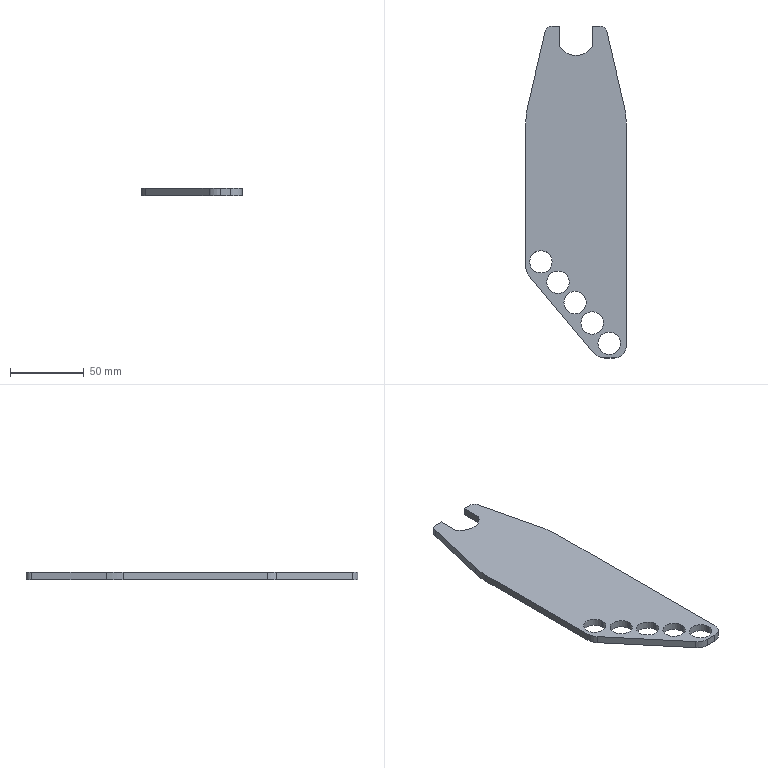Part | SolidWorks | features Fillet 5, ICE 4, Extrusion 1 | 1 solid | 30 faces | box 68 x 225 x 5 mm | volume 58604 mm3 | cylinder 18 | plane 12 | commonest cylinder face diameters 15.2 x10 10 x2 20 x2 100 x2 16 x1 26 x1
STEP:
#1=CARTESIAN_POINT('',(-8.24,-74.922,0.));
#2=VERTEX_POINT('',#1);
#3=CARTESIAN_POINT('',(6.96,-74.922,0.));
#4=VERTEX_POINT('',#3);
#5=CARTESIAN_POINT('',(-0.6404,-74.922,0.));
#6=DIRECTION('',(0.,0.,1.));
#7=DIRECTION('',(1.,0.,0.));
#8=AXIS2_PLACEMENT_3D('',#5,#6,#7);
#9=CIRCLE('',#8,7.6);
#10=EDGE_CURVE('',#2,#4,#9,.T.);
#11=ORIENTED_EDGE('',*,*,#10,.F.);
#12=CARTESIAN_POINT('',(-8.24,-74.922,5.));
#13=VERTEX_POINT('',#12);
#14=CARTESIAN_POINT('',(-8.24,-74.922,-3.));
#15=DIRECTION('',(0.,0.,1.));
#16=VECTOR('',#15,1000.);
#17=LINE('',#14,#16);
#18=EDGE_CURVE('',#2,#13,#17,.T.);
#19=ORIENTED_EDGE('',*,*,#18,.T.);
#20=CARTESIAN_POINT('',(6.96,-74.922,5.));
#21=VERTEX_POINT('',#20);
#22=CARTESIAN_POINT('',(-0.6404,-74.922,5.));
#23=DIRECTION('',(0.,0.,1.));
#24=DIRECTION('',(1.,0.,0.));
#25=AXIS2_PLACEMENT_3D('',#22,#23,#24);
#26=CIRCLE('',#25,7.6);
#27=EDGE_CURVE('',#13,#21,#26,.T.);
#28=ORIENTED_EDGE('',*,*,#27,.T.);
#29=CARTESIAN_POINT('',(6.96,-74.922,-3.));
#30=DIRECTION('',(0.,0.,1.));
#31=VECTOR('',#30,1000.);
#32=LINE('',#29,#31);
#33=EDGE_CURVE('',#4,#21,#32,.T.);
#34=ORIENTED_EDGE('',*,*,#33,.F.);
#35=EDGE_LOOP('',(#11,#19,#28,#34));
#36=FACE_OUTER_BOUND('',#35,.T.);
#37=CARTESIAN_POINT('',(-0.6404,-74.922,-3.));
#38=DIRECTION('',(0.,0.,1.));
#39=DIRECTION('',(1.,0.,0.));
#40=AXIS2_PLACEMENT_3D('',#37,#38,#39);
#41=CYLINDRICAL_SURFACE('',#40,7.6);
#42=ADVANCED_FACE('',(#36),#41,.F.);
#43=CARTESIAN_POINT('',(3.33,-88.711,0.));
#44=VERTEX_POINT('',#43);
#45=CARTESIAN_POINT('',(18.53,-88.711,0.));
#46=VERTEX_POINT('',#45);
#47=CARTESIAN_POINT('',(10.93,-88.711,0.));
#48=DIRECTION('',(0.,0.,1.));
#49=DIRECTION('',(1.,0.,0.));
#50=AXIS2_PLACEMENT_3D('',#47,#48,#49);
#51=CIRCLE('',#50,7.6);
#52=EDGE_CURVE('',#44,#46,#51,.T.);
#53=ORIENTED_EDGE('',*,*,#52,.F.);
#54=CARTESIAN_POINT('',(3.33,-88.711,5.));
#55=VERTEX_POINT('',#54);
#56=CARTESIAN_POINT('',(3.33,-88.711,-3.));
#57=DIRECTION('',(0.,0.,1.));
#58=VECTOR('',#57,1000.);
#59=LINE('',#56,#58);
#60=EDGE_CURVE('',#44,#55,#59,.T.);
#61=ORIENTED_EDGE('',*,*,#60,.T.);
#62=CARTESIAN_POINT('',(18.53,-88.711,5.));
#63=VERTEX_POINT('',#62);
#64=CARTESIAN_POINT('',(10.93,-88.711,5.));
#65=DIRECTION('',(0.,0.,1.));
#66=DIRECTION('',(1.,0.,0.));
#67=AXIS2_PLACEMENT_3D('',#64,#65,#66);
#68=CIRCLE('',#67,7.6);
#69=EDGE_CURVE('',#55,#63,#68,.T.);
#70=ORIENTED_EDGE('',*,*,#69,.T.);
#71=CARTESIAN_POINT('',(18.53,-88.711,-3.));
#72=DIRECTION('',(0.,0.,1.));
#73=VECTOR('',#72,1000.);
#74=LINE('',#71,#73);
#75=EDGE_CURVE('',#46,#63,#74,.T.);
#76=ORIENTED_EDGE('',*,*,#75,.F.);
#77=EDGE_LOOP('',(#53,#61,#70,#76));
#78=FACE_OUTER_BOUND('',#77,.T.);
#79=CARTESIAN_POINT('',(10.93,-88.711,-3.));
#80=DIRECTION('',(0.,0.,1.));
#81=DIRECTION('',(1.,0.,0.));
#82=AXIS2_PLACEMENT_3D('',#79,#80,#81);
#83=CYLINDRICAL_SURFACE('',#82,7.6);
#84=ADVANCED_FACE('',(#78),#83,.F.);
#85=CARTESIAN_POINT('',(-31.381,-47.345,0.));
#86=VERTEX_POINT('',#85);
#87=CARTESIAN_POINT('',(-16.181,-47.345,0.));
#88=VERTEX_POINT('',#87);
#89=CARTESIAN_POINT('',(-23.781,-47.345,0.));
#90=DIRECTION('',(0.,0.,1.));
#91=DIRECTION('',(1.,0.,0.));
#92=AXIS2_PLACEMENT_3D('',#89,#90,#91);
#93=CIRCLE('',#92,7.6);
#94=EDGE_CURVE('',#86,#88,#93,.T.);
#95=ORIENTED_EDGE('',*,*,#94,.F.);
#96=CARTESIAN_POINT('',(-31.381,-47.345,5.));
#97=VERTEX_POINT('',#96);
#98=CARTESIAN_POINT('',(-31.381,-47.345,-3.));
#99=DIRECTION('',(0.,0.,1.));
#100=VECTOR('',#99,1000.);
#101=LINE('',#98,#100);
#102=EDGE_CURVE('',#86,#97,#101,.T.);
#103=ORIENTED_EDGE('',*,*,#102,.T.);
#104=CARTESIAN_POINT('',(-16.181,-47.345,5.));
#105=VERTEX_POINT('',#104);
#106=CARTESIAN_POINT('',(-23.781,-47.345,5.));
#107=DIRECTION('',(0.,0.,1.));
#108=DIRECTION('',(1.,0.,0.));
#109=AXIS2_PLACEMENT_3D('',#106,#107,#108);
#110=CIRCLE('',#109,7.6);
#111=EDGE_CURVE('',#97,#105,#110,.T.);
#112=ORIENTED_EDGE('',*,*,#111,.T.);
#113=CARTESIAN_POINT('',(-16.181,-47.345,-3.));
#114=DIRECTION('',(0.,0.,1.));
#115=VECTOR('',#114,1000.);
#116=LINE('',#113,#115);
#117=EDGE_CURVE('',#88,#105,#116,.T.);
#118=ORIENTED_EDGE('',*,*,#117,.F.);
#119=EDGE_LOOP('',(#95,#103,#112,#118));
#120=FACE_OUTER_BOUND('',#119,.T.);
#121=CARTESIAN_POINT('',(-23.781,-47.345,-3.));
#122=DIRECTION('',(0.,0.,1.));
#123=DIRECTION('',(1.,0.,0.));
#124=AXIS2_PLACEMENT_3D('',#121,#122,#123);
#125=CYLINDRICAL_SURFACE('',#124,7.6);
#126=ADVANCED_FACE('',(#120),#125,.F.);
#127=CARTESIAN_POINT('',(-19.811,-61.134,0.));
#128=VERTEX_POINT('',#127);
#129=CARTESIAN_POINT('',(-4.611,-61.134,0.));
#130=VERTEX_POINT('',#129);
#131=CARTESIAN_POINT('',(-12.211,-61.134,0.));
#132=DIRECTION('',(0.,0.,1.));
#133=DIRECTION('',(1.,0.,0.));
#134=AXIS2_PLACEMENT_3D('',#131,#132,#133);
#135=CIRCLE('',#134,7.6);
#136=EDGE_CURVE('',#128,#130,#135,.T.);
#137=ORIENTED_EDGE('',*,*,#136,.F.);
#138=CARTESIAN_POINT('',(-19.811,-61.134,5.));
#139=VERTEX_POINT('',#138);
#140=CARTESIAN_POINT('',(-19.811,-61.134,-3.));
#141=DIRECTION('',(0.,0.,1.));
#142=VECTOR('',#141,1000.);
#143=LINE('',#140,#142);
#144=EDGE_CURVE('',#128,#139,#143,.T.);
#145=ORIENTED_EDGE('',*,*,#144,.T.);
#146=CARTESIAN_POINT('',(-4.611,-61.134,5.));
#147=VERTEX_POINT('',#146);
#148=CARTESIAN_POINT('',(-12.211,-61.134,5.));
#149=DIRECTION('',(0.,0.,1.));
#150=DIRECTION('',(1.,0.,0.));
#151=AXIS2_PLACEMENT_3D('',#148,#149,#150);
#152=CIRCLE('',#151,7.6);
#153=EDGE_CURVE('',#139,#147,#152,.T.);
#154=ORIENTED_EDGE('',*,*,#153,.T.);
#155=CARTESIAN_POINT('',(-4.611,-61.134,-3.));
#156=DIRECTION('',(0.,0.,1.));
#157=VECTOR('',#156,1000.);
#158=LINE('',#155,#157);
#159=EDGE_CURVE('',#130,#147,#158,.T.);
#160=ORIENTED_EDGE('',*,*,#159,.F.);
#161=EDGE_LOOP('',(#137,#145,#154,#160));
#162=FACE_OUTER_BOUND('',#161,.T.);
#163=CARTESIAN_POINT('',(-12.211,-61.134,-3.));
#164=DIRECTION('',(0.,0.,1.));
#165=DIRECTION('',(1.,0.,0.));
#166=AXIS2_PLACEMENT_3D('',#163,#164,#165);
#167=CYLINDRICAL_SURFACE('',#166,7.6);
#168=ADVANCED_FACE('',(#162),#167,.F.);
#169=CARTESIAN_POINT('',(14.9,-102.5,0.));
#170=VERTEX_POINT('',#169);
#171=CARTESIAN_POINT('',(30.1,-102.5,0.));
#172=VERTEX_POINT('',#171);
#173=CARTESIAN_POINT('',(22.5,-102.5,0.));
#174=DIRECTION('',(0.,0.,1.));
#175=DIRECTION('',(1.,0.,0.));
#176=AXIS2_PLACEMENT_3D('',#173,#174,#175);
#177=CIRCLE('',#176,7.6);
#178=EDGE_CURVE('',#170,#172,#177,.T.);
#179=ORIENTED_EDGE('',*,*,#178,.F.);
#180=CARTESIAN_POINT('',(14.9,-102.5,5.));
#181=VERTEX_POINT('',#180);
#182=CARTESIAN_POINT('',(14.9,-102.5,-3.));
#183=DIRECTION('',(0.,0.,1.));
#184=VECTOR('',#183,1000.);
#185=LINE('',#182,#184);
#186=EDGE_CURVE('',#170,#181,#185,.T.);
#187=ORIENTED_EDGE('',*,*,#186,.T.);
#188=CARTESIAN_POINT('',(30.1,-102.5,5.));
#189=VERTEX_POINT('',#188);
#190=CARTESIAN_POINT('',(22.5,-102.5,5.));
#191=DIRECTION('',(0.,0.,1.));
#192=DIRECTION('',(1.,0.,0.));
#193=AXIS2_PLACEMENT_3D('',#190,#191,#192);
#194=CIRCLE('',#193,7.6);
#195=EDGE_CURVE('',#181,#189,#194,.T.);
#196=ORIENTED_EDGE('',*,*,#195,.T.);
#197=CARTESIAN_POINT('',(30.1,-102.5,-3.));
#198=DIRECTION('',(0.,0.,1.));
#199=VECTOR('',#198,1000.);
#200=LINE('',#197,#199);
#201=EDGE_CURVE('',#172,#189,#200,.T.);
#202=ORIENTED_EDGE('',*,*,#201,.F.);
#203=EDGE_LOOP('',(#179,#187,#196,#202));
#204=FACE_OUTER_BOUND('',#203,.T.);
#205=CARTESIAN_POINT('',(22.5,-102.5,-3.));
#206=DIRECTION('',(0.,0.,1.));
#207=DIRECTION('',(1.,0.,0.));
#208=AXIS2_PLACEMENT_3D('',#205,#206,#207);
#209=CYLINDRICAL_SURFACE('',#208,7.6);
#210=ADVANCED_FACE('',(#204),#209,.F.);
#211=CARTESIAN_POINT('',(16.032,112.5,5.));
#212=VERTEX_POINT('',#211);
#213=CARTESIAN_POINT('',(11.,112.5,5.));
#214=VERTEX_POINT('',#213);
#215=CARTESIAN_POINT('',(-34.,112.5,5.));
#216=DIRECTION('',(-1.,0.,0.));
#217=VECTOR('',#216,1000.);
#218=LINE('',#215,#217);
#219=EDGE_CURVE('',#212,#214,#218,.T.);
#220=ORIENTED_EDGE('',*,*,#219,.F.);
#221=CARTESIAN_POINT('',(16.032,112.5,0.));
#222=VERTEX_POINT('',#221);
#223=CARTESIAN_POINT('',(16.032,112.5,5.));
#224=DIRECTION('',(0.,0.,-1.));
#225=VECTOR('',#224,1000.);
#226=LINE('',#223,#225);
#227=EDGE_CURVE('',#212,#222,#226,.T.);
#228=ORIENTED_EDGE('',*,*,#227,.T.);
#229=CARTESIAN_POINT('',(11.,112.5,0.));
#230=VERTEX_POINT('',#229);
#231=CARTESIAN_POINT('',(-34.,112.5,0.));
#232=DIRECTION('',(-1.,0.,0.));
#233=VECTOR('',#232,1000.);
#234=LINE('',#231,#233);
#235=EDGE_CURVE('',#222,#230,#234,.T.);
#236=ORIENTED_EDGE('',*,*,#235,.T.);
#237=CARTESIAN_POINT('',(11.,112.5,-3.));
#238=DIRECTION('',(0.,0.,1.));
#239=VECTOR('',#238,1000.);
#240=LINE('',#237,#239);
#241=EDGE_CURVE('',#230,#214,#240,.T.);
#242=ORIENTED_EDGE('',*,*,#241,.T.);
#243=EDGE_LOOP('',(#220,#228,#236,#242));
#244=FACE_OUTER_BOUND('',#243,.T.);
#245=CARTESIAN_POINT('',(-34.,112.5,5.));
#246=DIRECTION('',(0.,-1.,0.));
#247=DIRECTION('',(0.,0.,-1.));
#248=AXIS2_PLACEMENT_3D('',#245,#246,#247);
#249=PLANE('',#248);
#250=ADVANCED_FACE('',(#244),#249,.F.);
#251=CARTESIAN_POINT('',(34.,-104.5,0.));
#252=VERTEX_POINT('',#251);
#253=CARTESIAN_POINT('',(34.,46.744,0.));
#254=VERTEX_POINT('',#253);
#255=CARTESIAN_POINT('',(34.,112.5,0.));
#256=DIRECTION('',(0.,1.,0.));
#257=VECTOR('',#256,1000.);
#258=LINE('',#255,#257);
#259=EDGE_CURVE('',#252,#254,#258,.T.);
#260=ORIENTED_EDGE('',*,*,#259,.T.);
#261=CARTESIAN_POINT('',(34.,46.744,5.));
#262=VERTEX_POINT('',#261);
#263=CARTESIAN_POINT('',(34.,46.744,5.));
#264=DIRECTION('',(0.,0.,1.));
#265=VECTOR('',#264,1000.);
#266=LINE('',#263,#265);
#267=EDGE_CURVE('',#254,#262,#266,.T.);
#268=ORIENTED_EDGE('',*,*,#267,.T.);
#269=CARTESIAN_POINT('',(34.,-104.5,5.));
#270=VERTEX_POINT('',#269);
#271=CARTESIAN_POINT('',(34.,112.5,5.));
#272=DIRECTION('',(0.,1.,0.));
#273=VECTOR('',#272,1000.);
#274=LINE('',#271,#273);
#275=EDGE_CURVE('',#270,#262,#274,.T.);
#276=ORIENTED_EDGE('',*,*,#275,.F.);
#277=CARTESIAN_POINT('',(34.,-104.5,5.));
#278=DIRECTION('',(0.,0.,-1.));
#279=VECTOR('',#278,1000.);
#280=LINE('',#277,#279);
#281=EDGE_CURVE('',#270,#252,#280,.T.);
#282=ORIENTED_EDGE('',*,*,#281,.T.);
#283=EDGE_LOOP('',(#260,#268,#276,#282));
#284=FACE_OUTER_BOUND('',#283,.T.);
#285=CARTESIAN_POINT('',(34.,112.5,5.));
#286=DIRECTION('',(-1.,0.,0.));
#287=DIRECTION('',(0.,-1.,0.));
#288=AXIS2_PLACEMENT_3D('',#285,#286,#287);
#289=PLANE('',#288);
#290=ADVANCED_FACE('',(#284),#289,.F.);
#291=CARTESIAN_POINT('',(-11.,112.5,0.));
#292=VERTEX_POINT('',#291);
#293=CARTESIAN_POINT('',(-16.032,112.5,0.));
#294=VERTEX_POINT('',#293);
#295=CARTESIAN_POINT('',(-34.,112.5,0.));
#296=DIRECTION('',(-1.,0.,0.));
#297=VECTOR('',#296,1000.);
#298=LINE('',#295,#297);
#299=EDGE_CURVE('',#292,#294,#298,.T.);
#300=ORIENTED_EDGE('',*,*,#299,.T.);
#301=CARTESIAN_POINT('',(-16.032,112.5,5.));
#302=VERTEX_POINT('',#301);
#303=CARTESIAN_POINT('',(-16.032,112.5,5.));
#304=DIRECTION('',(0.,0.,1.));
#305=VECTOR('',#304,1000.);
#306=LINE('',#303,#305);
#307=EDGE_CURVE('',#294,#302,#306,.T.);
#308=ORIENTED_EDGE('',*,*,#307,.T.);
#309=CARTESIAN_POINT('',(-11.,112.5,5.));
#310=VERTEX_POINT('',#309);
#311=CARTESIAN_POINT('',(-34.,112.5,5.));
#312=DIRECTION('',(-1.,0.,0.));
#313=VECTOR('',#312,1000.);
#314=LINE('',#311,#313);
#315=EDGE_CURVE('',#310,#302,#314,.T.);
#316=ORIENTED_EDGE('',*,*,#315,.F.);
#317=CARTESIAN_POINT('',(-11.,112.5,-3.));
#318=DIRECTION('',(0.,0.,1.));
#319=VECTOR('',#318,1000.);
#320=LINE('',#317,#319);
#321=EDGE_CURVE('',#292,#310,#320,.T.);
#322=ORIENTED_EDGE('',*,*,#321,.F.);
#323=EDGE_LOOP('',(#300,#308,#316,#322));
#324=FACE_OUTER_BOUND('',#323,.T.);
#325=CARTESIAN_POINT('',(-34.,112.5,5.));
#326=DIRECTION('',(0.,-1.,0.));
#327=DIRECTION('',(0.,0.,-1.));
#328=AXIS2_PLACEMENT_3D('',#325,#326,#327);
#329=PLANE('',#328);
#330=ADVANCED_FACE('',(#324),#329,.F.);
#331=CARTESIAN_POINT('',(-34.,46.744,5.));
#332=VERTEX_POINT('',#331);
#333=CARTESIAN_POINT('',(-34.,-50.973,5.));
#334=VERTEX_POINT('',#333);
#335=CARTESIAN_POINT('',(-34.,112.5,5.));
#336=DIRECTION('',(0.,-1.,0.));
#337=VECTOR('',#336,1000.);
#338=LINE('',#335,#337);
#339=EDGE_CURVE('',#332,#334,#338,.T.);
#340=ORIENTED_EDGE('',*,*,#339,.F.);
#341=CARTESIAN_POINT('',(-34.,46.744,0.));
#342=VERTEX_POINT('',#341);
#343=CARTESIAN_POINT('',(-34.,46.744,5.));
#344=DIRECTION('',(0.,0.,-1.));
#345=VECTOR('',#344,1000.);
#346=LINE('',#343,#345);
#347=EDGE_CURVE('',#332,#342,#346,.T.);
#348=ORIENTED_EDGE('',*,*,#347,.T.);
#349=CARTESIAN_POINT('',(-34.,-50.973,0.));
#350=VERTEX_POINT('',#349);
#351=CARTESIAN_POINT('',(-34.,112.5,0.));
#352=DIRECTION('',(0.,-1.,0.));
#353=VECTOR('',#352,1000.);
#354=LINE('',#351,#353);
#355=EDGE_CURVE('',#342,#350,#354,.T.);
#356=ORIENTED_EDGE('',*,*,#355,.T.);
#357=CARTESIAN_POINT('',(-34.,-50.973,5.));
#358=DIRECTION('',(0.,0.,1.));
#359=VECTOR('',#358,1000.);
#360=LINE('',#357,#359);
#361=EDGE_CURVE('',#350,#334,#360,.T.);
#362=ORIENTED_EDGE('',*,*,#361,.T.);
#363=EDGE_LOOP('',(#340,#348,#356,#362));
#364=FACE_OUTER_BOUND('',#363,.T.);
#365=CARTESIAN_POINT('',(-34.,112.5,5.));
#366=DIRECTION('',(1.,0.,0.));
#367=DIRECTION('',(0.,1.,0.));
#368=AXIS2_PLACEMENT_3D('',#365,#366,#367);
#369=PLANE('',#368);
#370=ADVANCED_FACE('',(#364),#369,.F.);
#371=CARTESIAN_POINT('',(19.236,-112.5,5.));
#372=VERTEX_POINT('',#371);
#373=CARTESIAN_POINT('',(26.,-112.5,5.));
#374=VERTEX_POINT('',#373);
#375=CARTESIAN_POINT('',(-34.,-112.5,5.));
#376=DIRECTION('',(1.,0.,0.));
#377=VECTOR('',#376,1000.);
#378=LINE('',#375,#377);
#379=EDGE_CURVE('',#372,#374,#378,.T.);
#380=ORIENTED_EDGE('',*,*,#379,.F.);
#381=CARTESIAN_POINT('',(19.236,-112.5,0.));
#382=VERTEX_POINT('',#381);
#383=CARTESIAN_POINT('',(19.236,-112.5,5.));
#384=DIRECTION('',(0.,0.,-1.));
#385=VECTOR('',#384,1000.);
#386=LINE('',#383,#385);
#387=EDGE_CURVE('',#372,#382,#386,.T.);
#388=ORIENTED_EDGE('',*,*,#387,.T.);
#389=CARTESIAN_POINT('',(26.,-112.5,0.));
#390=VERTEX_POINT('',#389);
#391=CARTESIAN_POINT('',(-34.,-112.5,0.));
#392=DIRECTION('',(1.,0.,0.));
#393=VECTOR('',#392,1000.);
#394=LINE('',#391,#393);
#395=EDGE_CURVE('',#382,#390,#394,.T.);
#396=ORIENTED_EDGE('',*,*,#395,.T.);
#397=CARTESIAN_POINT('',(26.,-112.5,5.));
#398=DIRECTION('',(0.,0.,1.));
#399=VECTOR('',#398,1000.);
#400=LINE('',#397,#399);
#401=EDGE_CURVE('',#390,#374,#400,.T.);
#402=ORIENTED_EDGE('',*,*,#401,.T.);
#403=EDGE_LOOP('',(#380,#388,#396,#402));
#404=FACE_OUTER_BOUND('',#403,.T.);
#405=CARTESIAN_POINT('',(-34.,-112.5,5.));
#406=DIRECTION('',(0.,1.,0.));
#407=DIRECTION('',(0.,0.,1.));
#408=AXIS2_PLACEMENT_3D('',#405,#406,#407);
#409=PLANE('',#408);
#410=ADVANCED_FACE('',(#404),#409,.F.);
#411=ORIENTED_EDGE('',*,*,#275,.T.);
#412=CARTESIAN_POINT('',(32.692,58.105,5.));
#413=VERTEX_POINT('',#412);
#414=CARTESIAN_POINT('',(-16.,46.744,5.));
#415=DIRECTION('',(0.,0.,1.));
#416=DIRECTION('',(1.,0.,0.));
#417=AXIS2_PLACEMENT_3D('',#414,#415,#416);
#418=CIRCLE('',#417,50.);
#419=EDGE_CURVE('',#262,#413,#418,.T.);
#420=ORIENTED_EDGE('',*,*,#419,.T.);
#421=CARTESIAN_POINT('',(20.902,108.636,5.));
#422=VERTEX_POINT('',#421);
#423=CARTESIAN_POINT('',(20.,112.5,5.));
#424=DIRECTION('',(0.2272,-0.9738,0.));
#425=VECTOR('',#424,1000.);
#426=LINE('',#423,#425);
#427=EDGE_CURVE('',#422,#413,#426,.T.);
#428=ORIENTED_EDGE('',*,*,#427,.F.);
#429=CARTESIAN_POINT('',(16.032,107.5,5.));
#430=DIRECTION('',(0.,0.,1.));
#431=DIRECTION('',(1.,0.,0.));
#432=AXIS2_PLACEMENT_3D('',#429,#430,#431);
#433=CIRCLE('',#432,5.);
#434=EDGE_CURVE('',#422,#212,#433,.T.);
#435=ORIENTED_EDGE('',*,*,#434,.T.);
#436=ORIENTED_EDGE('',*,*,#219,.T.);
#437=CARTESIAN_POINT('',(11.,98.644,5.));
#438=VERTEX_POINT('',#437);
#439=CARTESIAN_POINT('',(11.,112.5,5.));
#440=DIRECTION('',(0.,1.,0.));
#441=VECTOR('',#440,1000.);
#442=LINE('',#439,#441);
#443=EDGE_CURVE('',#438,#214,#442,.T.);
#444=ORIENTED_EDGE('',*,*,#443,.F.);
#445=CARTESIAN_POINT('',(-11.,98.644,5.));
#446=VERTEX_POINT('',#445);
#447=CARTESIAN_POINT('',(0.,105.572,5.));
#448=DIRECTION('',(0.,0.,1.));
#449=DIRECTION('',(1.,0.,0.));
#450=AXIS2_PLACEMENT_3D('',#447,#448,#449);
#451=CIRCLE('',#450,13.);
#452=EDGE_CURVE('',#446,#438,#451,.T.);
#453=ORIENTED_EDGE('',*,*,#452,.F.);
#454=CARTESIAN_POINT('',(-11.,112.5,5.));
#455=DIRECTION('',(0.,-1.,0.));
#456=VECTOR('',#455,1000.);
#457=LINE('',#454,#456);
#458=EDGE_CURVE('',#310,#446,#457,.T.);
#459=ORIENTED_EDGE('',*,*,#458,.F.);
#460=ORIENTED_EDGE('',*,*,#315,.T.);
#461=CARTESIAN_POINT('',(-20.902,108.636,5.));
#462=VERTEX_POINT('',#461);
#463=CARTESIAN_POINT('',(-16.032,107.5,5.));
#464=DIRECTION('',(0.,0.,1.));
#465=DIRECTION('',(1.,0.,0.));
#466=AXIS2_PLACEMENT_3D('',#463,#464,#465);
#467=CIRCLE('',#466,5.);
#468=EDGE_CURVE('',#302,#462,#467,.T.);
#469=ORIENTED_EDGE('',*,*,#468,.T.);
#470=CARTESIAN_POINT('',(-32.692,58.105,5.));
#471=VERTEX_POINT('',#470);
#472=CARTESIAN_POINT('',(-20.,112.5,5.));
#473=DIRECTION('',(0.2272,0.9738,0.));
#474=VECTOR('',#473,1000.);
#475=LINE('',#472,#474);
#476=EDGE_CURVE('',#471,#462,#475,.T.);
#477=ORIENTED_EDGE('',*,*,#476,.F.);
#478=CARTESIAN_POINT('',(16.,46.744,5.));
#479=DIRECTION('',(0.,0.,1.));
#480=DIRECTION('',(1.,0.,0.));
#481=AXIS2_PLACEMENT_3D('',#478,#479,#480);
#482=CIRCLE('',#481,50.);
#483=EDGE_CURVE('',#471,#332,#482,.T.);
#484=ORIENTED_EDGE('',*,*,#483,.T.);
#485=ORIENTED_EDGE('',*,*,#339,.T.);
#486=CARTESIAN_POINT('',(-31.66,-57.401,5.));
#487=VERTEX_POINT('',#486);
#488=CARTESIAN_POINT('',(-24.,-50.973,5.));
#489=DIRECTION('',(0.,0.,1.));
#490=DIRECTION('',(1.,0.,0.));
#491=AXIS2_PLACEMENT_3D('',#488,#489,#490);
#492=CIRCLE('',#491,10.);
#493=EDGE_CURVE('',#334,#487,#492,.T.);
#494=ORIENTED_EDGE('',*,*,#493,.T.);
#495=CARTESIAN_POINT('',(11.576,-108.928,5.));
#496=VERTEX_POINT('',#495);
#497=CARTESIAN_POINT('',(14.573,-112.5,5.));
#498=DIRECTION('',(-0.6428,0.766,0.));
#499=VECTOR('',#498,1000.);
#500=LINE('',#497,#499);
#501=EDGE_CURVE('',#496,#487,#500,.T.);
#502=ORIENTED_EDGE('',*,*,#501,.F.);
#503=CARTESIAN_POINT('',(19.236,-102.5,5.));
#504=DIRECTION('',(0.,0.,1.));
#505=DIRECTION('',(1.,0.,0.));
#506=AXIS2_PLACEMENT_3D('',#503,#504,#505);
#507=CIRCLE('',#506,10.);
#508=EDGE_CURVE('',#496,#372,#507,.T.);
#509=ORIENTED_EDGE('',*,*,#508,.T.);
#510=ORIENTED_EDGE('',*,*,#379,.T.);
#511=CARTESIAN_POINT('',(26.,-104.5,5.));
#512=DIRECTION('',(0.,0.,1.));
#513=DIRECTION('',(1.,0.,0.));
#514=AXIS2_PLACEMENT_3D('',#511,#512,#513);
#515=CIRCLE('',#514,8.);
#516=EDGE_CURVE('',#374,#270,#515,.T.);
#517=ORIENTED_EDGE('',*,*,#516,.T.);
#518=EDGE_LOOP('',(#411,#420,#428,#435,#436,#444,#453,#459,#460,#469,#477,#484,#485,#494,#502,#509,#510,#517));
#519=FACE_OUTER_BOUND('',#518,.T.);
#520=CARTESIAN_POINT('',(-0.6404,-74.922,5.));
#521=DIRECTION('',(0.,0.,1.));
#522=DIRECTION('',(1.,0.,0.));
#523=AXIS2_PLACEMENT_3D('',#520,#521,#522);
#524=CIRCLE('',#523,7.6);
#525=EDGE_CURVE('',#21,#13,#524,.T.);
#526=ORIENTED_EDGE('',*,*,#525,.F.);
#527=ORIENTED_EDGE('',*,*,#27,.F.);
#528=EDGE_LOOP('',(#526,#527));
#529=FACE_BOUND('',#528,.T.);
#530=CARTESIAN_POINT('',(10.93,-88.711,5.));
#531=DIRECTION('',(0.,0.,1.));
#532=DIRECTION('',(1.,0.,0.));
#533=AXIS2_PLACEMENT_3D('',#530,#531,#532);
#534=CIRCLE('',#533,7.6);
#535=EDGE_CURVE('',#63,#55,#534,.T.);
#536=ORIENTED_EDGE('',*,*,#535,.F.);
#537=ORIENTED_EDGE('',*,*,#69,.F.);
#538=EDGE_LOOP('',(#536,#537));
#539=FACE_BOUND('',#538,.T.);
#540=CARTESIAN_POINT('',(-23.781,-47.345,5.));
#541=DIRECTION('',(0.,0.,1.));
#542=DIRECTION('',(1.,0.,0.));
#543=AXIS2_PLACEMENT_3D('',#540,#541,#542);
#544=CIRCLE('',#543,7.6);
#545=EDGE_CURVE('',#105,#97,#544,.T.);
#546=ORIENTED_EDGE('',*,*,#545,.F.);
#547=ORIENTED_EDGE('',*,*,#111,.F.);
#548=EDGE_LOOP('',(#546,#547));
#549=FACE_BOUND('',#548,.T.);
#550=CARTESIAN_POINT('',(-12.211,-61.134,5.));
#551=DIRECTION('',(0.,0.,1.));
#552=DIRECTION('',(1.,0.,0.));
#553=AXIS2_PLACEMENT_3D('',#550,#551,#552);
#554=CIRCLE('',#553,7.6);
#555=EDGE_CURVE('',#147,#139,#554,.T.);
#556=ORIENTED_EDGE('',*,*,#555,.F.);
#557=ORIENTED_EDGE('',*,*,#153,.F.);
#558=EDGE_LOOP('',(#556,#557));
#559=FACE_BOUND('',#558,.T.);
#560=CARTESIAN_POINT('',(22.5,-102.5,5.));
#561=DIRECTION('',(0.,0.,1.));
#562=DIRECTION('',(1.,0.,0.));
#563=AXIS2_PLACEMENT_3D('',#560,#561,#562);
#564=CIRCLE('',#563,7.6);
#565=EDGE_CURVE('',#189,#181,#564,.T.);
#566=ORIENTED_EDGE('',*,*,#565,.F.);
#567=ORIENTED_EDGE('',*,*,#195,.F.);
#568=EDGE_LOOP('',(#566,#567));
#569=FACE_BOUND('',#568,.T.);
#570=CARTESIAN_POINT('',(0.,0.,5.));
#571=DIRECTION('',(0.,0.,1.));
#572=DIRECTION('',(1.,0.,0.));
#573=AXIS2_PLACEMENT_3D('',#570,#571,#572);
#574=PLANE('',#573);
#575=ADVANCED_FACE('',(#519,#529,#539,#549,#559,#569),#574,.T.);
#576=CARTESIAN_POINT('',(-0.6404,-74.922,0.));
#577=DIRECTION('',(0.,0.,1.));
#578=DIRECTION('',(1.,0.,0.));
#579=AXIS2_PLACEMENT_3D('',#576,#577,#578);
#580=CIRCLE('',#579,7.6);
#581=EDGE_CURVE('',#4,#2,#580,.T.);
#582=ORIENTED_EDGE('',*,*,#581,.T.);
#583=ORIENTED_EDGE('',*,*,#10,.T.);
#584=EDGE_LOOP('',(#582,#583));
#585=FACE_BOUND('',#584,.T.);
#586=CARTESIAN_POINT('',(10.93,-88.711,0.));
#587=DIRECTION('',(0.,0.,1.));
#588=DIRECTION('',(1.,0.,0.));
#589=AXIS2_PLACEMENT_3D('',#586,#587,#588);
#590=CIRCLE('',#589,7.6);
#591=EDGE_CURVE('',#46,#44,#590,.T.);
#592=ORIENTED_EDGE('',*,*,#591,.T.);
#593=ORIENTED_EDGE('',*,*,#52,.T.);
#594=EDGE_LOOP('',(#592,#593));
#595=FACE_BOUND('',#594,.T.);
#596=CARTESIAN_POINT('',(-23.781,-47.345,0.));
#597=DIRECTION('',(0.,0.,1.));
#598=DIRECTION('',(1.,0.,0.));
#599=AXIS2_PLACEMENT_3D('',#596,#597,#598);
#600=CIRCLE('',#599,7.6);
#601=EDGE_CURVE('',#88,#86,#600,.T.);
#602=ORIENTED_EDGE('',*,*,#601,.T.);
#603=ORIENTED_EDGE('',*,*,#94,.T.);
#604=EDGE_LOOP('',(#602,#603));
#605=FACE_BOUND('',#604,.T.);
#606=CARTESIAN_POINT('',(-12.211,-61.134,0.));
#607=DIRECTION('',(0.,0.,1.));
#608=DIRECTION('',(1.,0.,0.));
#609=AXIS2_PLACEMENT_3D('',#606,#607,#608);
#610=CIRCLE('',#609,7.6);
#611=EDGE_CURVE('',#130,#128,#610,.T.);
#612=ORIENTED_EDGE('',*,*,#611,.T.);
#613=ORIENTED_EDGE('',*,*,#136,.T.);
#614=EDGE_LOOP('',(#612,#613));
#615=FACE_BOUND('',#614,.T.);
#616=CARTESIAN_POINT('',(22.5,-102.5,0.));
#617=DIRECTION('',(0.,0.,1.));
#618=DIRECTION('',(1.,0.,0.));
#619=AXIS2_PLACEMENT_3D('',#616,#617,#618);
#620=CIRCLE('',#619,7.6);
#621=EDGE_CURVE('',#172,#170,#620,.T.);
#622=ORIENTED_EDGE('',*,*,#621,.T.);
#623=ORIENTED_EDGE('',*,*,#178,.T.);
#624=EDGE_LOOP('',(#622,#623));
#625=FACE_BOUND('',#624,.T.);
#626=CARTESIAN_POINT('',(20.902,108.636,0.));
#627=VERTEX_POINT('',#626);
#628=CARTESIAN_POINT('',(32.692,58.105,0.));
#629=VERTEX_POINT('',#628);
#630=CARTESIAN_POINT('',(20.,112.5,0.));
#631=DIRECTION('',(0.2272,-0.9738,0.));
#632=VECTOR('',#631,1000.);
#633=LINE('',#630,#632);
#634=EDGE_CURVE('',#627,#629,#633,.T.);
#635=ORIENTED_EDGE('',*,*,#634,.T.);
#636=CARTESIAN_POINT('',(-16.,46.744,0.));
#637=DIRECTION('',(0.,0.,-1.));
#638=DIRECTION('',(1.,0.,0.));
#639=AXIS2_PLACEMENT_3D('',#636,#637,#638);
#640=CIRCLE('',#639,50.);
#641=EDGE_CURVE('',#629,#254,#640,.T.);
#642=ORIENTED_EDGE('',*,*,#641,.T.);
#643=ORIENTED_EDGE('',*,*,#259,.F.);
#644=CARTESIAN_POINT('',(26.,-104.5,0.));
#645=DIRECTION('',(0.,0.,-1.));
#646=DIRECTION('',(1.,0.,0.));
#647=AXIS2_PLACEMENT_3D('',#644,#645,#646);
#648=CIRCLE('',#647,8.);
#649=EDGE_CURVE('',#252,#390,#648,.T.);
#650=ORIENTED_EDGE('',*,*,#649,.T.);
#651=ORIENTED_EDGE('',*,*,#395,.F.);
#652=CARTESIAN_POINT('',(11.576,-108.928,0.));
#653=VERTEX_POINT('',#652);
#654=CARTESIAN_POINT('',(19.236,-102.5,0.));
#655=DIRECTION('',(0.,0.,-1.));
#656=DIRECTION('',(1.,0.,0.));
#657=AXIS2_PLACEMENT_3D('',#654,#655,#656);
#658=CIRCLE('',#657,10.);
#659=EDGE_CURVE('',#382,#653,#658,.T.);
#660=ORIENTED_EDGE('',*,*,#659,.T.);
#661=CARTESIAN_POINT('',(-31.66,-57.401,0.));
#662=VERTEX_POINT('',#661);
#663=CARTESIAN_POINT('',(14.573,-112.5,0.));
#664=DIRECTION('',(-0.6428,0.766,0.));
#665=VECTOR('',#664,1000.);
#666=LINE('',#663,#665);
#667=EDGE_CURVE('',#653,#662,#666,.T.);
#668=ORIENTED_EDGE('',*,*,#667,.T.);
#669=CARTESIAN_POINT('',(-24.,-50.973,0.));
#670=DIRECTION('',(0.,0.,-1.));
#671=DIRECTION('',(1.,0.,0.));
#672=AXIS2_PLACEMENT_3D('',#669,#670,#671);
#673=CIRCLE('',#672,10.);
#674=EDGE_CURVE('',#662,#350,#673,.T.);
#675=ORIENTED_EDGE('',*,*,#674,.T.);
#676=ORIENTED_EDGE('',*,*,#355,.F.);
#677=CARTESIAN_POINT('',(-32.692,58.105,0.));
#678=VERTEX_POINT('',#677);
#679=CARTESIAN_POINT('',(16.,46.744,0.));
#680=DIRECTION('',(0.,0.,-1.));
#681=DIRECTION('',(1.,0.,0.));
#682=AXIS2_PLACEMENT_3D('',#679,#680,#681);
#683=CIRCLE('',#682,50.);
#684=EDGE_CURVE('',#342,#678,#683,.T.);
#685=ORIENTED_EDGE('',*,*,#684,.T.);
#686=CARTESIAN_POINT('',(-20.902,108.636,0.));
#687=VERTEX_POINT('',#686);
#688=CARTESIAN_POINT('',(-20.,112.5,0.));
#689=DIRECTION('',(0.2272,0.9738,0.));
#690=VECTOR('',#689,1000.);
#691=LINE('',#688,#690);
#692=EDGE_CURVE('',#678,#687,#691,.T.);
#693=ORIENTED_EDGE('',*,*,#692,.T.);
#694=CARTESIAN_POINT('',(-16.032,107.5,0.));
#695=DIRECTION('',(0.,0.,-1.));
#696=DIRECTION('',(1.,0.,0.));
#697=AXIS2_PLACEMENT_3D('',#694,#695,#696);
#698=CIRCLE('',#697,5.);
#699=EDGE_CURVE('',#687,#294,#698,.T.);
#700=ORIENTED_EDGE('',*,*,#699,.T.);
#701=ORIENTED_EDGE('',*,*,#299,.F.);
#702=CARTESIAN_POINT('',(-11.,98.644,0.));
#703=VERTEX_POINT('',#702);
#704=CARTESIAN_POINT('',(-11.,0.,0.));
#705=DIRECTION('',(0.,-1.,0.));
#706=VECTOR('',#705,1000.);
#707=LINE('',#704,#706);
#708=EDGE_CURVE('',#292,#703,#707,.T.);
#709=ORIENTED_EDGE('',*,*,#708,.T.);
#710=CARTESIAN_POINT('',(11.,98.644,0.));
#711=VERTEX_POINT('',#710);
#712=CARTESIAN_POINT('',(0.,105.572,0.));
#713=DIRECTION('',(0.,0.,1.));
#714=DIRECTION('',(1.,0.,0.));
#715=AXIS2_PLACEMENT_3D('',#712,#713,#714);
#716=CIRCLE('',#715,13.);
#717=EDGE_CURVE('',#703,#711,#716,.T.);
#718=ORIENTED_EDGE('',*,*,#717,.T.);
#719=CARTESIAN_POINT('',(11.,0.,0.));
#720=DIRECTION('',(0.,1.,0.));
#721=VECTOR('',#720,1000.);
#722=LINE('',#719,#721);
#723=EDGE_CURVE('',#711,#230,#722,.T.);
#724=ORIENTED_EDGE('',*,*,#723,.T.);
#725=ORIENTED_EDGE('',*,*,#235,.F.);
#726=CARTESIAN_POINT('',(16.032,107.5,0.));
#727=DIRECTION('',(0.,0.,-1.));
#728=DIRECTION('',(1.,0.,0.));
#729=AXIS2_PLACEMENT_3D('',#726,#727,#728);
#730=CIRCLE('',#729,5.);
#731=EDGE_CURVE('',#222,#627,#730,.T.);
#732=ORIENTED_EDGE('',*,*,#731,.T.);
#733=EDGE_LOOP('',(#635,#642,#643,#650,#651,#660,#668,#675,#676,#685,#693,#700,#701,#709,#718,#724,#725,#732));
#734=FACE_OUTER_BOUND('',#733,.T.);
#735=CARTESIAN_POINT('',(0.,0.,0.));
#736=DIRECTION('',(0.,0.,1.));
#737=DIRECTION('',(1.,0.,0.));
#738=AXIS2_PLACEMENT_3D('',#735,#736,#737);
#739=PLANE('',#738);
#740=ADVANCED_FACE('',(#585,#595,#605,#615,#625,#734),#739,.F.);
#741=ORIENTED_EDGE('',*,*,#186,.F.);
#742=ORIENTED_EDGE('',*,*,#621,.F.);
#743=ORIENTED_EDGE('',*,*,#201,.T.);
#744=ORIENTED_EDGE('',*,*,#565,.T.);
#745=EDGE_LOOP('',(#741,#742,#743,#744));
#746=FACE_OUTER_BOUND('',#745,.T.);
#747=CARTESIAN_POINT('',(22.5,-102.5,-3.));
#748=DIRECTION('',(0.,0.,1.));
#749=DIRECTION('',(1.,0.,0.));
#750=AXIS2_PLACEMENT_3D('',#747,#748,#749);
#751=CYLINDRICAL_SURFACE('',#750,7.6);
#752=ADVANCED_FACE('',(#746),#751,.F.);
#753=ORIENTED_EDGE('',*,*,#144,.F.);
#754=ORIENTED_EDGE('',*,*,#611,.F.);
#755=ORIENTED_EDGE('',*,*,#159,.T.);
#756=ORIENTED_EDGE('',*,*,#555,.T.);
#757=EDGE_LOOP('',(#753,#754,#755,#756));
#758=FACE_OUTER_BOUND('',#757,.T.);
#759=CARTESIAN_POINT('',(-12.211,-61.134,-3.));
#760=DIRECTION('',(0.,0.,1.));
#761=DIRECTION('',(1.,0.,0.));
#762=AXIS2_PLACEMENT_3D('',#759,#760,#761);
#763=CYLINDRICAL_SURFACE('',#762,7.6);
#764=ADVANCED_FACE('',(#758),#763,.F.);
#765=ORIENTED_EDGE('',*,*,#102,.F.);
#766=ORIENTED_EDGE('',*,*,#601,.F.);
#767=ORIENTED_EDGE('',*,*,#117,.T.);
#768=ORIENTED_EDGE('',*,*,#545,.T.);
#769=EDGE_LOOP('',(#765,#766,#767,#768));
#770=FACE_OUTER_BOUND('',#769,.T.);
#771=CARTESIAN_POINT('',(-23.781,-47.345,-3.));
#772=DIRECTION('',(0.,0.,1.));
#773=DIRECTION('',(1.,0.,0.));
#774=AXIS2_PLACEMENT_3D('',#771,#772,#773);
#775=CYLINDRICAL_SURFACE('',#774,7.6);
#776=ADVANCED_FACE('',(#770),#775,.F.);
#777=ORIENTED_EDGE('',*,*,#60,.F.);
#778=ORIENTED_EDGE('',*,*,#591,.F.);
#779=ORIENTED_EDGE('',*,*,#75,.T.);
#780=ORIENTED_EDGE('',*,*,#535,.T.);
#781=EDGE_LOOP('',(#777,#778,#779,#780));
#782=FACE_OUTER_BOUND('',#781,.T.);
#783=CARTESIAN_POINT('',(10.93,-88.711,-3.));
#784=DIRECTION('',(0.,0.,1.));
#785=DIRECTION('',(1.,0.,0.));
#786=AXIS2_PLACEMENT_3D('',#783,#784,#785);
#787=CYLINDRICAL_SURFACE('',#786,7.6);
#788=ADVANCED_FACE('',(#782),#787,.F.);
#789=ORIENTED_EDGE('',*,*,#18,.F.);
#790=ORIENTED_EDGE('',*,*,#581,.F.);
#791=ORIENTED_EDGE('',*,*,#33,.T.);
#792=ORIENTED_EDGE('',*,*,#525,.T.);
#793=EDGE_LOOP('',(#789,#790,#791,#792));
#794=FACE_OUTER_BOUND('',#793,.T.);
#795=CARTESIAN_POINT('',(-0.6404,-74.922,-3.));
#796=DIRECTION('',(0.,0.,1.));
#797=DIRECTION('',(1.,0.,0.));
#798=AXIS2_PLACEMENT_3D('',#795,#796,#797);
#799=CYLINDRICAL_SURFACE('',#798,7.6);
#800=ADVANCED_FACE('',(#794),#799,.F.);
#801=ORIENTED_EDGE('',*,*,#516,.F.);
#802=ORIENTED_EDGE('',*,*,#401,.F.);
#803=ORIENTED_EDGE('',*,*,#649,.F.);
#804=ORIENTED_EDGE('',*,*,#281,.F.);
#805=EDGE_LOOP('',(#801,#802,#803,#804));
#806=FACE_OUTER_BOUND('',#805,.T.);
#807=CARTESIAN_POINT('',(26.,-104.5,5.));
#808=DIRECTION('',(0.,0.,-1.));
#809=DIRECTION('',(-1.,0.,0.));
#810=AXIS2_PLACEMENT_3D('',#807,#808,#809);
#811=CYLINDRICAL_SURFACE('',#810,8.);
#812=ADVANCED_FACE('',(#806),#811,.T.);
#813=ORIENTED_EDGE('',*,*,#501,.T.);
#814=CARTESIAN_POINT('',(-31.66,-57.401,0.));
#815=DIRECTION('',(0.,0.,-1.));
#816=VECTOR('',#815,1000.);
#817=LINE('',#814,#816);
#818=EDGE_CURVE('',#487,#662,#817,.T.);
#819=ORIENTED_EDGE('',*,*,#818,.T.);
#820=ORIENTED_EDGE('',*,*,#667,.F.);
#821=CARTESIAN_POINT('',(11.576,-108.928,0.));
#822=DIRECTION('',(0.,0.,1.));
#823=VECTOR('',#822,1000.);
#824=LINE('',#821,#823);
#825=EDGE_CURVE('',#653,#496,#824,.T.);
#826=ORIENTED_EDGE('',*,*,#825,.T.);
#827=EDGE_LOOP('',(#813,#819,#820,#826));
#828=FACE_OUTER_BOUND('',#827,.T.);
#829=CARTESIAN_POINT('',(14.573,-112.5,0.));
#830=DIRECTION('',(0.766,0.6428,0.));
#831=DIRECTION('',(-0.6428,0.766,0.));
#832=AXIS2_PLACEMENT_3D('',#829,#830,#831);
#833=PLANE('',#832);
#834=ADVANCED_FACE('',(#828),#833,.F.);
#835=ORIENTED_EDGE('',*,*,#659,.F.);
#836=ORIENTED_EDGE('',*,*,#387,.F.);
#837=ORIENTED_EDGE('',*,*,#508,.F.);
#838=ORIENTED_EDGE('',*,*,#825,.F.);
#839=EDGE_LOOP('',(#835,#836,#837,#838));
#840=FACE_OUTER_BOUND('',#839,.T.);
#841=CARTESIAN_POINT('',(19.236,-102.5,0.));
#842=DIRECTION('',(0.,0.,1.));
#843=DIRECTION('',(1.,0.,0.));
#844=AXIS2_PLACEMENT_3D('',#841,#842,#843);
#845=CYLINDRICAL_SURFACE('',#844,10.);
#846=ADVANCED_FACE('',(#840),#845,.T.);
#847=CARTESIAN_POINT('',(11.,98.644,-3.));
#848=DIRECTION('',(0.,0.,1.));
#849=VECTOR('',#848,1000.);
#850=LINE('',#847,#849);
#851=EDGE_CURVE('',#711,#438,#850,.T.);
#852=ORIENTED_EDGE('',*,*,#851,.T.);
#853=ORIENTED_EDGE('',*,*,#443,.T.);
#854=ORIENTED_EDGE('',*,*,#241,.F.);
#855=ORIENTED_EDGE('',*,*,#723,.F.);
#856=EDGE_LOOP('',(#852,#853,#854,#855));
#857=FACE_OUTER_BOUND('',#856,.T.);
#858=CARTESIAN_POINT('',(11.,112.5,-3.));
#859=DIRECTION('',(1.,0.,0.));
#860=DIRECTION('',(0.,0.,-1.));
#861=AXIS2_PLACEMENT_3D('',#858,#859,#860);
#862=PLANE('',#861);
#863=ADVANCED_FACE('',(#857),#862,.F.);
#864=CARTESIAN_POINT('',(-11.,98.644,-3.));
#865=DIRECTION('',(0.,0.,1.));
#866=VECTOR('',#865,1000.);
#867=LINE('',#864,#866);
#868=EDGE_CURVE('',#703,#446,#867,.T.);
#869=ORIENTED_EDGE('',*,*,#868,.T.);
#870=ORIENTED_EDGE('',*,*,#452,.T.);
#871=ORIENTED_EDGE('',*,*,#851,.F.);
#872=ORIENTED_EDGE('',*,*,#717,.F.);
#873=EDGE_LOOP('',(#869,#870,#871,#872));
#874=FACE_OUTER_BOUND('',#873,.T.);
#875=CARTESIAN_POINT('',(0.,105.572,-3.));
#876=DIRECTION('',(0.,0.,1.));
#877=DIRECTION('',(1.,0.,0.));
#878=AXIS2_PLACEMENT_3D('',#875,#876,#877);
#879=CYLINDRICAL_SURFACE('',#878,13.);
#880=ADVANCED_FACE('',(#874),#879,.F.);
#881=ORIENTED_EDGE('',*,*,#321,.T.);
#882=ORIENTED_EDGE('',*,*,#458,.T.);
#883=ORIENTED_EDGE('',*,*,#868,.F.);
#884=ORIENTED_EDGE('',*,*,#708,.F.);
#885=EDGE_LOOP('',(#881,#882,#883,#884));
#886=FACE_OUTER_BOUND('',#885,.T.);
#887=CARTESIAN_POINT('',(-11.,112.5,-3.));
#888=DIRECTION('',(-1.,0.,0.));
#889=DIRECTION('',(0.,-1.,0.));
#890=AXIS2_PLACEMENT_3D('',#887,#888,#889);
#891=PLANE('',#890);
#892=ADVANCED_FACE('',(#886),#891,.F.);
#893=ORIENTED_EDGE('',*,*,#674,.F.);
#894=ORIENTED_EDGE('',*,*,#818,.F.);
#895=ORIENTED_EDGE('',*,*,#493,.F.);
#896=ORIENTED_EDGE('',*,*,#361,.F.);
#897=EDGE_LOOP('',(#893,#894,#895,#896));
#898=FACE_OUTER_BOUND('',#897,.T.);
#899=CARTESIAN_POINT('',(-24.,-50.973,5.));
#900=DIRECTION('',(0.,0.,1.));
#901=DIRECTION('',(1.,0.,0.));
#902=AXIS2_PLACEMENT_3D('',#899,#900,#901);
#903=CYLINDRICAL_SURFACE('',#902,10.);
#904=ADVANCED_FACE('',(#898),#903,.T.);
#905=ORIENTED_EDGE('',*,*,#427,.T.);
#906=CARTESIAN_POINT('',(32.692,58.105,0.));
#907=DIRECTION('',(0.,0.,-1.));
#908=VECTOR('',#907,1000.);
#909=LINE('',#906,#908);
#910=EDGE_CURVE('',#413,#629,#909,.T.);
#911=ORIENTED_EDGE('',*,*,#910,.T.);
#912=ORIENTED_EDGE('',*,*,#634,.F.);
#913=CARTESIAN_POINT('',(20.902,108.636,0.));
#914=DIRECTION('',(0.,0.,1.));
#915=VECTOR('',#914,1000.);
#916=LINE('',#913,#915);
#917=EDGE_CURVE('',#627,#422,#916,.T.);
#918=ORIENTED_EDGE('',*,*,#917,.T.);
#919=EDGE_LOOP('',(#905,#911,#912,#918));
#920=FACE_OUTER_BOUND('',#919,.T.);
#921=CARTESIAN_POINT('',(20.,112.5,0.));
#922=DIRECTION('',(-0.9738,-0.2272,0.));
#923=DIRECTION('',(0.2272,-0.9738,0.));
#924=AXIS2_PLACEMENT_3D('',#921,#922,#923);
#925=PLANE('',#924);
#926=ADVANCED_FACE('',(#920),#925,.F.);
#927=ORIENTED_EDGE('',*,*,#692,.F.);
#928=CARTESIAN_POINT('',(-32.692,58.105,0.));
#929=DIRECTION('',(0.,0.,1.));
#930=VECTOR('',#929,1000.);
#931=LINE('',#928,#930);
#932=EDGE_CURVE('',#678,#471,#931,.T.);
#933=ORIENTED_EDGE('',*,*,#932,.T.);
#934=ORIENTED_EDGE('',*,*,#476,.T.);
#935=CARTESIAN_POINT('',(-20.902,108.636,0.));
#936=DIRECTION('',(0.,0.,-1.));
#937=VECTOR('',#936,1000.);
#938=LINE('',#935,#937);
#939=EDGE_CURVE('',#462,#687,#938,.T.);
#940=ORIENTED_EDGE('',*,*,#939,.T.);
#941=EDGE_LOOP('',(#927,#933,#934,#940));
#942=FACE_OUTER_BOUND('',#941,.T.);
#943=CARTESIAN_POINT('',(-20.,112.5,0.));
#944=DIRECTION('',(0.9738,-0.2272,0.));
#945=DIRECTION('',(0.2272,0.9738,0.));
#946=AXIS2_PLACEMENT_3D('',#943,#944,#945);
#947=PLANE('',#946);
#948=ADVANCED_FACE('',(#942),#947,.F.);
#949=ORIENTED_EDGE('',*,*,#731,.F.);
#950=ORIENTED_EDGE('',*,*,#227,.F.);
#951=ORIENTED_EDGE('',*,*,#434,.F.);
#952=ORIENTED_EDGE('',*,*,#917,.F.);
#953=EDGE_LOOP('',(#949,#950,#951,#952));
#954=FACE_OUTER_BOUND('',#953,.T.);
#955=CARTESIAN_POINT('',(16.032,107.5,0.));
#956=DIRECTION('',(0.,0.,1.));
#957=DIRECTION('',(1.,0.,0.));
#958=AXIS2_PLACEMENT_3D('',#955,#956,#957);
#959=CYLINDRICAL_SURFACE('',#958,5.);
#960=ADVANCED_FACE('',(#954),#959,.T.);
#961=ORIENTED_EDGE('',*,*,#699,.F.);
#962=ORIENTED_EDGE('',*,*,#939,.F.);
#963=ORIENTED_EDGE('',*,*,#468,.F.);
#964=ORIENTED_EDGE('',*,*,#307,.F.);
#965=EDGE_LOOP('',(#961,#962,#963,#964));
#966=FACE_OUTER_BOUND('',#965,.T.);
#967=CARTESIAN_POINT('',(-16.032,107.5,5.));
#968=DIRECTION('',(0.,0.,1.));
#969=DIRECTION('',(1.,0.,0.));
#970=AXIS2_PLACEMENT_3D('',#967,#968,#969);
#971=CYLINDRICAL_SURFACE('',#970,5.);
#972=ADVANCED_FACE('',(#966),#971,.T.);
#973=ORIENTED_EDGE('',*,*,#641,.F.);
#974=ORIENTED_EDGE('',*,*,#910,.F.);
#975=ORIENTED_EDGE('',*,*,#419,.F.);
#976=ORIENTED_EDGE('',*,*,#267,.F.);
#977=EDGE_LOOP('',(#973,#974,#975,#976));
#978=FACE_OUTER_BOUND('',#977,.T.);
#979=CARTESIAN_POINT('',(-16.,46.744,5.));
#980=DIRECTION('',(0.,0.,1.));
#981=DIRECTION('',(1.,0.,0.));
#982=AXIS2_PLACEMENT_3D('',#979,#980,#981);
#983=CYLINDRICAL_SURFACE('',#982,50.);
#984=ADVANCED_FACE('',(#978),#983,.T.);
#985=ORIENTED_EDGE('',*,*,#684,.F.);
#986=ORIENTED_EDGE('',*,*,#347,.F.);
#987=ORIENTED_EDGE('',*,*,#483,.F.);
#988=ORIENTED_EDGE('',*,*,#932,.F.);
#989=EDGE_LOOP('',(#985,#986,#987,#988));
#990=FACE_OUTER_BOUND('',#989,.T.);
#991=CARTESIAN_POINT('',(16.,46.744,0.));
#992=DIRECTION('',(0.,0.,1.));
#993=DIRECTION('',(1.,0.,0.));
#994=AXIS2_PLACEMENT_3D('',#991,#992,#993);
#995=CYLINDRICAL_SURFACE('',#994,50.);
#996=ADVANCED_FACE('',(#990),#995,.T.);
#997=CLOSED_SHELL('',(#42,#84,#126,#168,#210,#250,#290,#330,#370,#410,#575,#740,#752,#764,#776,#788,#800,#812,#834,#846,#863,#880,#892,#904,#926,#948,#960,#972,#984,#996));
#998=MANIFOLD_SOLID_BREP('',#997);
#999=CARTESIAN_POINT('',(0.,0.,0.));
#1000=DIRECTION('',(0.,0.,1.));
#1001=DIRECTION('',(1.,0.,0.));
#1002=AXIS2_PLACEMENT_3D('',#999,#1000,#1001);
#1003=(LENGTH_UNIT()NAMED_UNIT(*)SI_UNIT(.MILLI.,.METRE.));
#1004=UNCERTAINTY_MEASURE_WITH_UNIT(LENGTH_MEASURE(0.00001),#1003,'','');
#1005=(NAMED_UNIT(*)PLANE_ANGLE_UNIT()SI_UNIT($,.RADIAN.));
#1006=(NAMED_UNIT(*)SI_UNIT($,.STERADIAN.)SOLID_ANGLE_UNIT());
#1007=(GEOMETRIC_REPRESENTATION_CONTEXT(3)GLOBAL_UNCERTAINTY_ASSIGNED_CONTEXT((#1004))GLOBAL_UNIT_ASSIGNED_CONTEXT((#1003,#1005,#1006))REPRESENTATION_CONTEXT('',''));
#1008=ADVANCED_BREP_SHAPE_REPRESENTATION('',(#998,#1002),#1007);